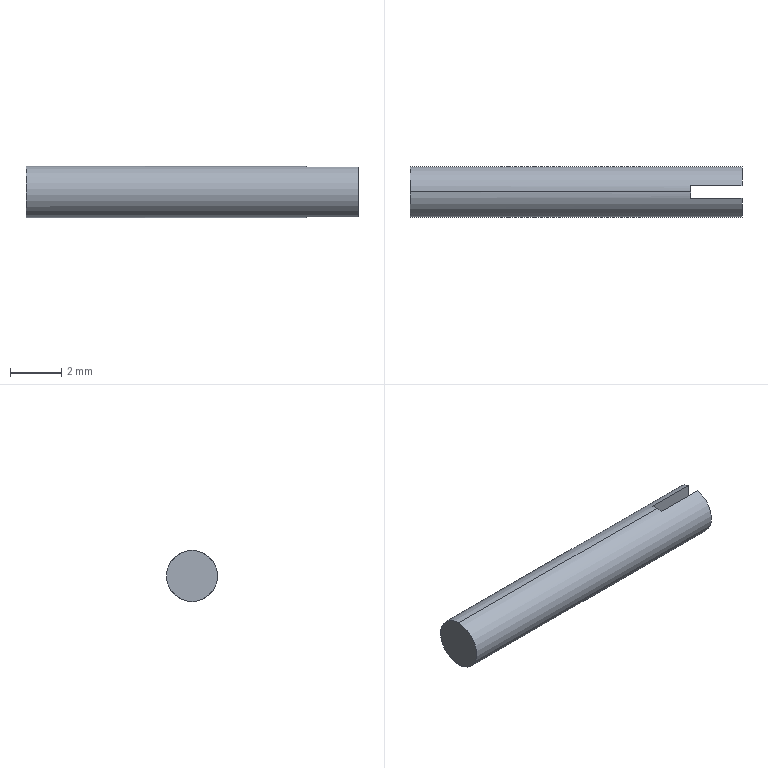Part | SolidWorks | features Extrusion 1, ICE 1 | 1 solid | 8 faces | box 13 x 2 x 2 mm | volume 38.862 mm3 | plane 6 | cylinder 2 | commonest cylinder face diameters 2 x2
STEP:
#1=CARTESIAN_POINT('',(11.,0.25,-0.9682));
#2=VERTEX_POINT('',#1);
#3=CARTESIAN_POINT('',(11.,0.,-1.));
#4=VERTEX_POINT('',#3);
#5=CARTESIAN_POINT('',(11.,0.,0.));
#6=DIRECTION('',(-1.,0.,0.));
#7=DIRECTION('',(0.,0.,1.));
#8=AXIS2_PLACEMENT_3D('',#5,#6,#7);
#9=CIRCLE('',#8,1.);
#10=EDGE_CURVE('',#2,#4,#9,.T.);
#11=ORIENTED_EDGE('',*,*,#10,.T.);
#12=CARTESIAN_POINT('',(0.,0.,-1.));
#13=VERTEX_POINT('',#12);
#14=CARTESIAN_POINT('',(13.,0.,-1.));
#15=DIRECTION('',(-1.,0.,0.));
#16=VECTOR('',#15,1000.);
#17=LINE('',#14,#16);
#18=EDGE_CURVE('',#4,#13,#17,.T.);
#19=ORIENTED_EDGE('',*,*,#18,.T.);
#20=CARTESIAN_POINT('',(0.,0.,1.));
#21=VERTEX_POINT('',#20);
#22=CARTESIAN_POINT('',(0.,0.,0.));
#23=DIRECTION('',(1.,0.,0.));
#24=DIRECTION('',(0.,0.,-1.));
#25=AXIS2_PLACEMENT_3D('',#22,#23,#24);
#26=CIRCLE('',#25,1.);
#27=EDGE_CURVE('',#13,#21,#26,.T.);
#28=ORIENTED_EDGE('',*,*,#27,.T.);
#29=CARTESIAN_POINT('',(11.,0.,1.));
#30=VERTEX_POINT('',#29);
#31=CARTESIAN_POINT('',(13.,0.,1.));
#32=DIRECTION('',(-1.,0.,0.));
#33=VECTOR('',#32,1000.);
#34=LINE('',#31,#33);
#35=EDGE_CURVE('',#30,#21,#34,.T.);
#36=ORIENTED_EDGE('',*,*,#35,.F.);
#37=CARTESIAN_POINT('',(11.,0.25,0.9682));
#38=VERTEX_POINT('',#37);
#39=CARTESIAN_POINT('',(11.,0.,0.));
#40=DIRECTION('',(-1.,0.,0.));
#41=DIRECTION('',(0.,0.,1.));
#42=AXIS2_PLACEMENT_3D('',#39,#40,#41);
#43=CIRCLE('',#42,1.);
#44=EDGE_CURVE('',#30,#38,#43,.T.);
#45=ORIENTED_EDGE('',*,*,#44,.T.);
#46=CARTESIAN_POINT('',(13.,0.25,0.9682));
#47=VERTEX_POINT('',#46);
#48=CARTESIAN_POINT('',(13.,0.25,0.9682));
#49=DIRECTION('',(1.,0.,0.));
#50=VECTOR('',#49,1000.);
#51=LINE('',#48,#50);
#52=EDGE_CURVE('',#38,#47,#51,.T.);
#53=ORIENTED_EDGE('',*,*,#52,.T.);
#54=CARTESIAN_POINT('',(13.,0.25,-0.9682));
#55=VERTEX_POINT('',#54);
#56=CARTESIAN_POINT('',(13.,0.,0.));
#57=DIRECTION('',(1.,0.,0.));
#58=DIRECTION('',(0.,0.,-1.));
#59=AXIS2_PLACEMENT_3D('',#56,#57,#58);
#60=CIRCLE('',#59,1.);
#61=EDGE_CURVE('',#55,#47,#60,.T.);
#62=ORIENTED_EDGE('',*,*,#61,.F.);
#63=CARTESIAN_POINT('',(13.,0.25,-0.9682));
#64=DIRECTION('',(-1.,0.,0.));
#65=VECTOR('',#64,1000.);
#66=LINE('',#63,#65);
#67=EDGE_CURVE('',#55,#2,#66,.T.);
#68=ORIENTED_EDGE('',*,*,#67,.T.);
#69=EDGE_LOOP('',(#11,#19,#28,#36,#45,#53,#62,#68));
#70=FACE_OUTER_BOUND('',#69,.T.);
#71=CARTESIAN_POINT('',(13.,0.,0.));
#72=DIRECTION('',(-1.,0.,0.));
#73=DIRECTION('',(0.,0.,1.));
#74=AXIS2_PLACEMENT_3D('',#71,#72,#73);
#75=CYLINDRICAL_SURFACE('',#74,1.);
#76=ADVANCED_FACE('',(#70),#75,.T.);
#77=CARTESIAN_POINT('',(13.,-0.25,0.9682));
#78=VERTEX_POINT('',#77);
#79=CARTESIAN_POINT('',(13.,-0.25,-0.9682));
#80=VERTEX_POINT('',#79);
#81=CARTESIAN_POINT('',(13.,-0.25,0.));
#82=DIRECTION('',(0.,0.,-1.));
#83=VECTOR('',#82,1000.);
#84=LINE('',#81,#83);
#85=EDGE_CURVE('',#78,#80,#84,.T.);
#86=ORIENTED_EDGE('',*,*,#85,.F.);
#87=CARTESIAN_POINT('',(13.,0.,0.));
#88=DIRECTION('',(1.,0.,0.));
#89=DIRECTION('',(0.,0.,-1.));
#90=AXIS2_PLACEMENT_3D('',#87,#88,#89);
#91=CIRCLE('',#90,1.);
#92=EDGE_CURVE('',#78,#80,#91,.T.);
#93=ORIENTED_EDGE('',*,*,#92,.T.);
#94=EDGE_LOOP('',(#86,#93));
#95=FACE_OUTER_BOUND('',#94,.T.);
#96=CARTESIAN_POINT('',(13.,0.,0.));
#97=DIRECTION('',(1.,0.,0.));
#98=DIRECTION('',(0.,0.,-1.));
#99=AXIS2_PLACEMENT_3D('',#96,#97,#98);
#100=PLANE('',#99);
#101=ADVANCED_FACE('',(#95),#100,.T.);
#102=ORIENTED_EDGE('',*,*,#18,.F.);
#103=CARTESIAN_POINT('',(11.,-0.25,-0.9682));
#104=VERTEX_POINT('',#103);
#105=CARTESIAN_POINT('',(11.,0.,0.));
#106=DIRECTION('',(-1.,0.,0.));
#107=DIRECTION('',(0.,0.,1.));
#108=AXIS2_PLACEMENT_3D('',#105,#106,#107);
#109=CIRCLE('',#108,1.);
#110=EDGE_CURVE('',#4,#104,#109,.T.);
#111=ORIENTED_EDGE('',*,*,#110,.T.);
#112=CARTESIAN_POINT('',(13.,-0.25,-0.9682));
#113=DIRECTION('',(1.,0.,0.));
#114=VECTOR('',#113,1000.);
#115=LINE('',#112,#114);
#116=EDGE_CURVE('',#104,#80,#115,.T.);
#117=ORIENTED_EDGE('',*,*,#116,.T.);
#118=ORIENTED_EDGE('',*,*,#92,.F.);
#119=CARTESIAN_POINT('',(11.,-0.25,0.9682));
#120=VERTEX_POINT('',#119);
#121=CARTESIAN_POINT('',(13.,-0.25,0.9682));
#122=DIRECTION('',(-1.,0.,0.));
#123=VECTOR('',#122,1000.);
#124=LINE('',#121,#123);
#125=EDGE_CURVE('',#78,#120,#124,.T.);
#126=ORIENTED_EDGE('',*,*,#125,.T.);
#127=CARTESIAN_POINT('',(11.,0.,0.));
#128=DIRECTION('',(-1.,0.,0.));
#129=DIRECTION('',(0.,0.,1.));
#130=AXIS2_PLACEMENT_3D('',#127,#128,#129);
#131=CIRCLE('',#130,1.);
#132=EDGE_CURVE('',#120,#30,#131,.T.);
#133=ORIENTED_EDGE('',*,*,#132,.T.);
#134=ORIENTED_EDGE('',*,*,#35,.T.);
#135=CARTESIAN_POINT('',(0.,0.,0.));
#136=DIRECTION('',(1.,0.,0.));
#137=DIRECTION('',(0.,0.,-1.));
#138=AXIS2_PLACEMENT_3D('',#135,#136,#137);
#139=CIRCLE('',#138,1.);
#140=EDGE_CURVE('',#21,#13,#139,.T.);
#141=ORIENTED_EDGE('',*,*,#140,.T.);
#142=EDGE_LOOP('',(#102,#111,#117,#118,#126,#133,#134,#141));
#143=FACE_OUTER_BOUND('',#142,.T.);
#144=CARTESIAN_POINT('',(13.,0.,0.));
#145=DIRECTION('',(-1.,0.,0.));
#146=DIRECTION('',(0.,0.,1.));
#147=AXIS2_PLACEMENT_3D('',#144,#145,#146);
#148=CYLINDRICAL_SURFACE('',#147,1.);
#149=ADVANCED_FACE('',(#143),#148,.T.);
#150=CARTESIAN_POINT('',(13.,0.25,0.));
#151=DIRECTION('',(0.,0.,1.));
#152=VECTOR('',#151,1000.);
#153=LINE('',#150,#152);
#154=EDGE_CURVE('',#55,#47,#153,.T.);
#155=ORIENTED_EDGE('',*,*,#154,.F.);
#156=ORIENTED_EDGE('',*,*,#61,.T.);
#157=EDGE_LOOP('',(#155,#156));
#158=FACE_OUTER_BOUND('',#157,.T.);
#159=CARTESIAN_POINT('',(13.,0.,0.));
#160=DIRECTION('',(1.,0.,0.));
#161=DIRECTION('',(0.,0.,-1.));
#162=AXIS2_PLACEMENT_3D('',#159,#160,#161);
#163=PLANE('',#162);
#164=ADVANCED_FACE('',(#158),#163,.T.);
#165=ORIENTED_EDGE('',*,*,#140,.F.);
#166=ORIENTED_EDGE('',*,*,#27,.F.);
#167=EDGE_LOOP('',(#165,#166));
#168=FACE_OUTER_BOUND('',#167,.T.);
#169=CARTESIAN_POINT('',(0.,0.,0.));
#170=DIRECTION('',(1.,0.,0.));
#171=DIRECTION('',(0.,0.,-1.));
#172=AXIS2_PLACEMENT_3D('',#169,#170,#171);
#173=PLANE('',#172);
#174=ADVANCED_FACE('',(#168),#173,.F.);
#175=CARTESIAN_POINT('',(11.,0.25,1.278));
#176=DIRECTION('',(0.,0.,1.));
#177=VECTOR('',#176,1000.);
#178=LINE('',#175,#177);
#179=EDGE_CURVE('',#2,#38,#178,.T.);
#180=ORIENTED_EDGE('',*,*,#179,.T.);
#181=ORIENTED_EDGE('',*,*,#44,.F.);
#182=ORIENTED_EDGE('',*,*,#132,.F.);
#183=CARTESIAN_POINT('',(11.,-0.25,1.278));
#184=DIRECTION('',(0.,0.,-1.));
#185=VECTOR('',#184,1000.);
#186=LINE('',#183,#185);
#187=EDGE_CURVE('',#120,#104,#186,.T.);
#188=ORIENTED_EDGE('',*,*,#187,.T.);
#189=ORIENTED_EDGE('',*,*,#110,.F.);
#190=ORIENTED_EDGE('',*,*,#10,.F.);
#191=EDGE_LOOP('',(#180,#181,#182,#188,#189,#190));
#192=FACE_OUTER_BOUND('',#191,.T.);
#193=CARTESIAN_POINT('',(11.,0.,0.));
#194=DIRECTION('',(-1.,0.,0.));
#195=DIRECTION('',(0.,0.,1.));
#196=AXIS2_PLACEMENT_3D('',#193,#194,#195);
#197=PLANE('',#196);
#198=ADVANCED_FACE('',(#192),#197,.F.);
#199=ORIENTED_EDGE('',*,*,#85,.T.);
#200=ORIENTED_EDGE('',*,*,#116,.F.);
#201=ORIENTED_EDGE('',*,*,#187,.F.);
#202=ORIENTED_EDGE('',*,*,#125,.F.);
#203=EDGE_LOOP('',(#199,#200,#201,#202));
#204=FACE_OUTER_BOUND('',#203,.T.);
#205=CARTESIAN_POINT('',(11.,-0.25,1.278));
#206=DIRECTION('',(0.,-1.,0.));
#207=DIRECTION('',(0.,0.,-1.));
#208=AXIS2_PLACEMENT_3D('',#205,#206,#207);
#209=PLANE('',#208);
#210=ADVANCED_FACE('',(#204),#209,.F.);
#211=ORIENTED_EDGE('',*,*,#154,.T.);
#212=ORIENTED_EDGE('',*,*,#52,.F.);
#213=ORIENTED_EDGE('',*,*,#179,.F.);
#214=ORIENTED_EDGE('',*,*,#67,.F.);
#215=EDGE_LOOP('',(#211,#212,#213,#214));
#216=FACE_OUTER_BOUND('',#215,.T.);
#217=CARTESIAN_POINT('',(11.,0.25,1.278));
#218=DIRECTION('',(0.,1.,0.));
#219=DIRECTION('',(0.,0.,1.));
#220=AXIS2_PLACEMENT_3D('',#217,#218,#219);
#221=PLANE('',#220);
#222=ADVANCED_FACE('',(#216),#221,.F.);
#223=CLOSED_SHELL('',(#76,#101,#149,#164,#174,#198,#210,#222));
#224=MANIFOLD_SOLID_BREP('',#223);
#225=CARTESIAN_POINT('',(0.,0.,0.));
#226=DIRECTION('',(0.,0.,1.));
#227=DIRECTION('',(1.,0.,0.));
#228=AXIS2_PLACEMENT_3D('',#225,#226,#227);
#229=(LENGTH_UNIT()NAMED_UNIT(*)SI_UNIT(.MILLI.,.METRE.));
#230=UNCERTAINTY_MEASURE_WITH_UNIT(LENGTH_MEASURE(0.00001),#229,'','');
#231=(NAMED_UNIT(*)PLANE_ANGLE_UNIT()SI_UNIT($,.RADIAN.));
#232=(NAMED_UNIT(*)SI_UNIT($,.STERADIAN.)SOLID_ANGLE_UNIT());
#233=(GEOMETRIC_REPRESENTATION_CONTEXT(3)GLOBAL_UNCERTAINTY_ASSIGNED_CONTEXT((#230))GLOBAL_UNIT_ASSIGNED_CONTEXT((#229,#231,#232))REPRESENTATION_CONTEXT('',''));
#234=ADVANCED_BREP_SHAPE_REPRESENTATION('',(#224,#228),#233);